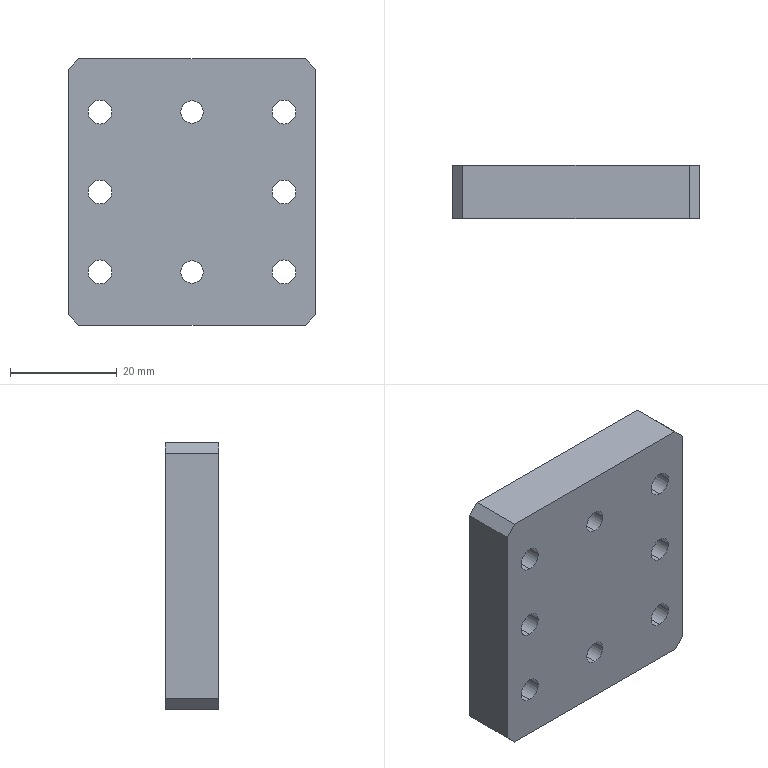Part | SolidWorks | features HoleWzd 2, Chamfer 1, Extrusion 1 | 1 solid | 44 faces | box 46.5 x 10 x 50 mm | volume 20990 mm3 | cylinder 28 | plane 16 | commonest cylinder face diameters 4.5 x12 8 x12 4.2 x4
STEP:
#1=CARTESIAN_POINT('',(0.,0.,-17.1));
#2=VERTEX_POINT('',#1);
#3=CARTESIAN_POINT('',(0.,0.,-12.9));
#4=VERTEX_POINT('',#3);
#5=CARTESIAN_POINT('',(0.,0.,-15.));
#6=DIRECTION('',(0.,1.,0.));
#7=DIRECTION('',(0.,0.,1.));
#8=AXIS2_PLACEMENT_3D('',#5,#6,#7);
#9=CIRCLE('',#8,2.1);
#10=EDGE_CURVE('',#2,#4,#9,.T.);
#11=ORIENTED_EDGE('',*,*,#10,.F.);
#12=CARTESIAN_POINT('',(0.,10.,-17.1));
#13=VERTEX_POINT('',#12);
#14=CARTESIAN_POINT('',(0.,10.,-17.1));
#15=DIRECTION('',(0.,1.,0.));
#16=VECTOR('',#15,1000.);
#17=LINE('',#14,#16);
#18=EDGE_CURVE('',#2,#13,#17,.T.);
#19=ORIENTED_EDGE('',*,*,#18,.T.);
#20=CARTESIAN_POINT('',(0.,10.,-12.9));
#21=VERTEX_POINT('',#20);
#22=CARTESIAN_POINT('',(0.,10.,-15.));
#23=DIRECTION('',(0.,1.,0.));
#24=DIRECTION('',(0.,0.,1.));
#25=AXIS2_PLACEMENT_3D('',#22,#23,#24);
#26=CIRCLE('',#25,2.1);
#27=EDGE_CURVE('',#13,#21,#26,.T.);
#28=ORIENTED_EDGE('',*,*,#27,.T.);
#29=CARTESIAN_POINT('',(0.,10.,-12.9));
#30=DIRECTION('',(0.,1.,0.));
#31=VECTOR('',#30,1000.);
#32=LINE('',#29,#31);
#33=EDGE_CURVE('',#4,#21,#32,.T.);
#34=ORIENTED_EDGE('',*,*,#33,.F.);
#35=EDGE_LOOP('',(#11,#19,#28,#34));
#36=FACE_OUTER_BOUND('',#35,.T.);
#37=CARTESIAN_POINT('',(0.,10.,-15.));
#38=DIRECTION('',(0.,1.,0.));
#39=DIRECTION('',(0.,0.,1.));
#40=AXIS2_PLACEMENT_3D('',#37,#38,#39);
#41=CYLINDRICAL_SURFACE('',#40,2.1);
#42=ADVANCED_FACE('',(#36),#41,.F.);
#43=CARTESIAN_POINT('',(0.,0.,12.9));
#44=VERTEX_POINT('',#43);
#45=CARTESIAN_POINT('',(0.,0.,17.1));
#46=VERTEX_POINT('',#45);
#47=CARTESIAN_POINT('',(0.,0.,15.));
#48=DIRECTION('',(0.,1.,0.));
#49=DIRECTION('',(0.,0.,1.));
#50=AXIS2_PLACEMENT_3D('',#47,#48,#49);
#51=CIRCLE('',#50,2.1);
#52=EDGE_CURVE('',#44,#46,#51,.T.);
#53=ORIENTED_EDGE('',*,*,#52,.F.);
#54=CARTESIAN_POINT('',(0.,10.,12.9));
#55=VERTEX_POINT('',#54);
#56=CARTESIAN_POINT('',(0.,10.,12.9));
#57=DIRECTION('',(0.,1.,0.));
#58=VECTOR('',#57,1000.);
#59=LINE('',#56,#58);
#60=EDGE_CURVE('',#44,#55,#59,.T.);
#61=ORIENTED_EDGE('',*,*,#60,.T.);
#62=CARTESIAN_POINT('',(0.,10.,17.1));
#63=VERTEX_POINT('',#62);
#64=CARTESIAN_POINT('',(0.,10.,15.));
#65=DIRECTION('',(0.,1.,0.));
#66=DIRECTION('',(0.,0.,1.));
#67=AXIS2_PLACEMENT_3D('',#64,#65,#66);
#68=CIRCLE('',#67,2.1);
#69=EDGE_CURVE('',#55,#63,#68,.T.);
#70=ORIENTED_EDGE('',*,*,#69,.T.);
#71=CARTESIAN_POINT('',(0.,10.,17.1));
#72=DIRECTION('',(0.,1.,0.));
#73=VECTOR('',#72,1000.);
#74=LINE('',#71,#73);
#75=EDGE_CURVE('',#46,#63,#74,.T.);
#76=ORIENTED_EDGE('',*,*,#75,.F.);
#77=EDGE_LOOP('',(#53,#61,#70,#76));
#78=FACE_OUTER_BOUND('',#77,.T.);
#79=CARTESIAN_POINT('',(0.,10.,15.));
#80=DIRECTION('',(0.,1.,0.));
#81=DIRECTION('',(0.,0.,1.));
#82=AXIS2_PLACEMENT_3D('',#79,#80,#81);
#83=CYLINDRICAL_SURFACE('',#82,2.1);
#84=ADVANCED_FACE('',(#78),#83,.F.);
#85=CARTESIAN_POINT('',(17.25,5.4,11.));
#86=VERTEX_POINT('',#85);
#87=CARTESIAN_POINT('',(17.25,5.4,19.));
#88=VERTEX_POINT('',#87);
#89=CARTESIAN_POINT('',(17.25,5.4,15.));
#90=DIRECTION('',(0.,1.,0.));
#91=DIRECTION('',(0.,0.,1.));
#92=AXIS2_PLACEMENT_3D('',#89,#90,#91);
#93=CIRCLE('',#92,4.);
#94=EDGE_CURVE('',#86,#88,#93,.T.);
#95=ORIENTED_EDGE('',*,*,#94,.F.);
#96=CARTESIAN_POINT('',(17.25,10.,11.));
#97=VERTEX_POINT('',#96);
#98=CARTESIAN_POINT('',(17.25,10.,11.));
#99=DIRECTION('',(0.,1.,0.));
#100=VECTOR('',#99,1000.);
#101=LINE('',#98,#100);
#102=EDGE_CURVE('',#86,#97,#101,.T.);
#103=ORIENTED_EDGE('',*,*,#102,.T.);
#104=CARTESIAN_POINT('',(17.25,10.,19.));
#105=VERTEX_POINT('',#104);
#106=CARTESIAN_POINT('',(17.25,10.,15.));
#107=DIRECTION('',(0.,1.,0.));
#108=DIRECTION('',(0.,0.,1.));
#109=AXIS2_PLACEMENT_3D('',#106,#107,#108);
#110=CIRCLE('',#109,4.);
#111=EDGE_CURVE('',#97,#105,#110,.T.);
#112=ORIENTED_EDGE('',*,*,#111,.T.);
#113=CARTESIAN_POINT('',(17.25,10.,19.));
#114=DIRECTION('',(0.,1.,0.));
#115=VECTOR('',#114,1000.);
#116=LINE('',#113,#115);
#117=EDGE_CURVE('',#88,#105,#116,.T.);
#118=ORIENTED_EDGE('',*,*,#117,.F.);
#119=EDGE_LOOP('',(#95,#103,#112,#118));
#120=FACE_OUTER_BOUND('',#119,.T.);
#121=CARTESIAN_POINT('',(17.25,10.,15.));
#122=DIRECTION('',(0.,1.,0.));
#123=DIRECTION('',(0.,0.,1.));
#124=AXIS2_PLACEMENT_3D('',#121,#122,#123);
#125=CYLINDRICAL_SURFACE('',#124,4.);
#126=ADVANCED_FACE('',(#120),#125,.F.);
#127=CARTESIAN_POINT('',(17.25,0.,12.75));
#128=VERTEX_POINT('',#127);
#129=CARTESIAN_POINT('',(17.25,0.,17.25));
#130=VERTEX_POINT('',#129);
#131=CARTESIAN_POINT('',(17.25,0.,15.));
#132=DIRECTION('',(0.,1.,0.));
#133=DIRECTION('',(0.,0.,1.));
#134=AXIS2_PLACEMENT_3D('',#131,#132,#133);
#135=CIRCLE('',#134,2.25);
#136=EDGE_CURVE('',#128,#130,#135,.T.);
#137=ORIENTED_EDGE('',*,*,#136,.F.);
#138=CARTESIAN_POINT('',(17.25,5.4,12.75));
#139=VERTEX_POINT('',#138);
#140=CARTESIAN_POINT('',(17.25,10.,12.75));
#141=DIRECTION('',(0.,1.,0.));
#142=VECTOR('',#141,1000.);
#143=LINE('',#140,#142);
#144=EDGE_CURVE('',#128,#139,#143,.T.);
#145=ORIENTED_EDGE('',*,*,#144,.T.);
#146=CARTESIAN_POINT('',(17.25,5.4,17.25));
#147=VERTEX_POINT('',#146);
#148=CARTESIAN_POINT('',(17.25,5.4,15.));
#149=DIRECTION('',(0.,1.,0.));
#150=DIRECTION('',(0.,0.,1.));
#151=AXIS2_PLACEMENT_3D('',#148,#149,#150);
#152=CIRCLE('',#151,2.25);
#153=EDGE_CURVE('',#139,#147,#152,.T.);
#154=ORIENTED_EDGE('',*,*,#153,.T.);
#155=CARTESIAN_POINT('',(17.25,10.,17.25));
#156=DIRECTION('',(0.,1.,0.));
#157=VECTOR('',#156,1000.);
#158=LINE('',#155,#157);
#159=EDGE_CURVE('',#130,#147,#158,.T.);
#160=ORIENTED_EDGE('',*,*,#159,.F.);
#161=EDGE_LOOP('',(#137,#145,#154,#160));
#162=FACE_OUTER_BOUND('',#161,.T.);
#163=CARTESIAN_POINT('',(17.25,10.,15.));
#164=DIRECTION('',(0.,1.,0.));
#165=DIRECTION('',(0.,0.,1.));
#166=AXIS2_PLACEMENT_3D('',#163,#164,#165);
#167=CYLINDRICAL_SURFACE('',#166,2.25);
#168=ADVANCED_FACE('',(#162),#167,.F.);
#169=CARTESIAN_POINT('',(17.25,5.4,-4.));
#170=VERTEX_POINT('',#169);
#171=CARTESIAN_POINT('',(17.25,5.4,4.));
#172=VERTEX_POINT('',#171);
#173=CARTESIAN_POINT('',(17.25,5.4,0.));
#174=DIRECTION('',(0.,1.,0.));
#175=DIRECTION('',(0.,0.,1.));
#176=AXIS2_PLACEMENT_3D('',#173,#174,#175);
#177=CIRCLE('',#176,4.);
#178=EDGE_CURVE('',#170,#172,#177,.T.);
#179=ORIENTED_EDGE('',*,*,#178,.F.);
#180=CARTESIAN_POINT('',(17.25,10.,-4.));
#181=VERTEX_POINT('',#180);
#182=CARTESIAN_POINT('',(17.25,10.,-4.));
#183=DIRECTION('',(0.,1.,0.));
#184=VECTOR('',#183,1000.);
#185=LINE('',#182,#184);
#186=EDGE_CURVE('',#170,#181,#185,.T.);
#187=ORIENTED_EDGE('',*,*,#186,.T.);
#188=CARTESIAN_POINT('',(17.25,10.,4.));
#189=VERTEX_POINT('',#188);
#190=CARTESIAN_POINT('',(17.25,10.,0.));
#191=DIRECTION('',(0.,1.,0.));
#192=DIRECTION('',(0.,0.,1.));
#193=AXIS2_PLACEMENT_3D('',#190,#191,#192);
#194=CIRCLE('',#193,4.);
#195=EDGE_CURVE('',#181,#189,#194,.T.);
#196=ORIENTED_EDGE('',*,*,#195,.T.);
#197=CARTESIAN_POINT('',(17.25,10.,4.));
#198=DIRECTION('',(0.,1.,0.));
#199=VECTOR('',#198,1000.);
#200=LINE('',#197,#199);
#201=EDGE_CURVE('',#172,#189,#200,.T.);
#202=ORIENTED_EDGE('',*,*,#201,.F.);
#203=EDGE_LOOP('',(#179,#187,#196,#202));
#204=FACE_OUTER_BOUND('',#203,.T.);
#205=CARTESIAN_POINT('',(17.25,10.,0.));
#206=DIRECTION('',(0.,1.,0.));
#207=DIRECTION('',(0.,0.,1.));
#208=AXIS2_PLACEMENT_3D('',#205,#206,#207);
#209=CYLINDRICAL_SURFACE('',#208,4.);
#210=ADVANCED_FACE('',(#204),#209,.F.);
#211=CARTESIAN_POINT('',(17.25,0.,-2.25));
#212=VERTEX_POINT('',#211);
#213=CARTESIAN_POINT('',(17.25,0.,2.25));
#214=VERTEX_POINT('',#213);
#215=CARTESIAN_POINT('',(17.25,0.,0.));
#216=DIRECTION('',(0.,1.,0.));
#217=DIRECTION('',(0.,0.,1.));
#218=AXIS2_PLACEMENT_3D('',#215,#216,#217);
#219=CIRCLE('',#218,2.25);
#220=EDGE_CURVE('',#212,#214,#219,.T.);
#221=ORIENTED_EDGE('',*,*,#220,.F.);
#222=CARTESIAN_POINT('',(17.25,5.4,-2.25));
#223=VERTEX_POINT('',#222);
#224=CARTESIAN_POINT('',(17.25,10.,-2.25));
#225=DIRECTION('',(0.,1.,0.));
#226=VECTOR('',#225,1000.);
#227=LINE('',#224,#226);
#228=EDGE_CURVE('',#212,#223,#227,.T.);
#229=ORIENTED_EDGE('',*,*,#228,.T.);
#230=CARTESIAN_POINT('',(17.25,5.4,2.25));
#231=VERTEX_POINT('',#230);
#232=CARTESIAN_POINT('',(17.25,5.4,0.));
#233=DIRECTION('',(0.,1.,0.));
#234=DIRECTION('',(0.,0.,1.));
#235=AXIS2_PLACEMENT_3D('',#232,#233,#234);
#236=CIRCLE('',#235,2.25);
#237=EDGE_CURVE('',#223,#231,#236,.T.);
#238=ORIENTED_EDGE('',*,*,#237,.T.);
#239=CARTESIAN_POINT('',(17.25,10.,2.25));
#240=DIRECTION('',(0.,1.,0.));
#241=VECTOR('',#240,1000.);
#242=LINE('',#239,#241);
#243=EDGE_CURVE('',#214,#231,#242,.T.);
#244=ORIENTED_EDGE('',*,*,#243,.F.);
#245=EDGE_LOOP('',(#221,#229,#238,#244));
#246=FACE_OUTER_BOUND('',#245,.T.);
#247=CARTESIAN_POINT('',(17.25,10.,0.));
#248=DIRECTION('',(0.,1.,0.));
#249=DIRECTION('',(0.,0.,1.));
#250=AXIS2_PLACEMENT_3D('',#247,#248,#249);
#251=CYLINDRICAL_SURFACE('',#250,2.25);
#252=ADVANCED_FACE('',(#246),#251,.F.);
#253=CARTESIAN_POINT('',(17.25,5.4,-19.));
#254=VERTEX_POINT('',#253);
#255=CARTESIAN_POINT('',(17.25,5.4,-11.));
#256=VERTEX_POINT('',#255);
#257=CARTESIAN_POINT('',(17.25,5.4,-15.));
#258=DIRECTION('',(0.,1.,0.));
#259=DIRECTION('',(0.,0.,1.));
#260=AXIS2_PLACEMENT_3D('',#257,#258,#259);
#261=CIRCLE('',#260,4.);
#262=EDGE_CURVE('',#254,#256,#261,.T.);
#263=ORIENTED_EDGE('',*,*,#262,.F.);
#264=CARTESIAN_POINT('',(17.25,10.,-19.));
#265=VERTEX_POINT('',#264);
#266=CARTESIAN_POINT('',(17.25,10.,-19.));
#267=DIRECTION('',(0.,1.,0.));
#268=VECTOR('',#267,1000.);
#269=LINE('',#266,#268);
#270=EDGE_CURVE('',#254,#265,#269,.T.);
#271=ORIENTED_EDGE('',*,*,#270,.T.);
#272=CARTESIAN_POINT('',(17.25,10.,-11.));
#273=VERTEX_POINT('',#272);
#274=CARTESIAN_POINT('',(17.25,10.,-15.));
#275=DIRECTION('',(0.,1.,0.));
#276=DIRECTION('',(0.,0.,1.));
#277=AXIS2_PLACEMENT_3D('',#274,#275,#276);
#278=CIRCLE('',#277,4.);
#279=EDGE_CURVE('',#265,#273,#278,.T.);
#280=ORIENTED_EDGE('',*,*,#279,.T.);
#281=CARTESIAN_POINT('',(17.25,10.,-11.));
#282=DIRECTION('',(0.,1.,0.));
#283=VECTOR('',#282,1000.);
#284=LINE('',#281,#283);
#285=EDGE_CURVE('',#256,#273,#284,.T.);
#286=ORIENTED_EDGE('',*,*,#285,.F.);
#287=EDGE_LOOP('',(#263,#271,#280,#286));
#288=FACE_OUTER_BOUND('',#287,.T.);
#289=CARTESIAN_POINT('',(17.25,10.,-15.));
#290=DIRECTION('',(0.,1.,0.));
#291=DIRECTION('',(0.,0.,1.));
#292=AXIS2_PLACEMENT_3D('',#289,#290,#291);
#293=CYLINDRICAL_SURFACE('',#292,4.);
#294=ADVANCED_FACE('',(#288),#293,.F.);
#295=CARTESIAN_POINT('',(17.25,0.,-17.25));
#296=VERTEX_POINT('',#295);
#297=CARTESIAN_POINT('',(17.25,0.,-12.75));
#298=VERTEX_POINT('',#297);
#299=CARTESIAN_POINT('',(17.25,0.,-15.));
#300=DIRECTION('',(0.,1.,0.));
#301=DIRECTION('',(0.,0.,1.));
#302=AXIS2_PLACEMENT_3D('',#299,#300,#301);
#303=CIRCLE('',#302,2.25);
#304=EDGE_CURVE('',#296,#298,#303,.T.);
#305=ORIENTED_EDGE('',*,*,#304,.F.);
#306=CARTESIAN_POINT('',(17.25,5.4,-17.25));
#307=VERTEX_POINT('',#306);
#308=CARTESIAN_POINT('',(17.25,10.,-17.25));
#309=DIRECTION('',(0.,1.,0.));
#310=VECTOR('',#309,1000.);
#311=LINE('',#308,#310);
#312=EDGE_CURVE('',#296,#307,#311,.T.);
#313=ORIENTED_EDGE('',*,*,#312,.T.);
#314=CARTESIAN_POINT('',(17.25,5.4,-12.75));
#315=VERTEX_POINT('',#314);
#316=CARTESIAN_POINT('',(17.25,5.4,-15.));
#317=DIRECTION('',(0.,1.,0.));
#318=DIRECTION('',(0.,0.,1.));
#319=AXIS2_PLACEMENT_3D('',#316,#317,#318);
#320=CIRCLE('',#319,2.25);
#321=EDGE_CURVE('',#307,#315,#320,.T.);
#322=ORIENTED_EDGE('',*,*,#321,.T.);
#323=CARTESIAN_POINT('',(17.25,10.,-12.75));
#324=DIRECTION('',(0.,1.,0.));
#325=VECTOR('',#324,1000.);
#326=LINE('',#323,#325);
#327=EDGE_CURVE('',#298,#315,#326,.T.);
#328=ORIENTED_EDGE('',*,*,#327,.F.);
#329=EDGE_LOOP('',(#305,#313,#322,#328));
#330=FACE_OUTER_BOUND('',#329,.T.);
#331=CARTESIAN_POINT('',(17.25,10.,-15.));
#332=DIRECTION('',(0.,1.,0.));
#333=DIRECTION('',(0.,0.,1.));
#334=AXIS2_PLACEMENT_3D('',#331,#332,#333);
#335=CYLINDRICAL_SURFACE('',#334,2.25);
#336=ADVANCED_FACE('',(#330),#335,.F.);
#337=CARTESIAN_POINT('',(-17.25,5.4,-19.));
#338=VERTEX_POINT('',#337);
#339=CARTESIAN_POINT('',(-17.25,5.4,-11.));
#340=VERTEX_POINT('',#339);
#341=CARTESIAN_POINT('',(-17.25,5.4,-15.));
#342=DIRECTION('',(0.,1.,0.));
#343=DIRECTION('',(0.,0.,1.));
#344=AXIS2_PLACEMENT_3D('',#341,#342,#343);
#345=CIRCLE('',#344,4.);
#346=EDGE_CURVE('',#338,#340,#345,.T.);
#347=ORIENTED_EDGE('',*,*,#346,.F.);
#348=CARTESIAN_POINT('',(-17.25,10.,-19.));
#349=VERTEX_POINT('',#348);
#350=CARTESIAN_POINT('',(-17.25,10.,-19.));
#351=DIRECTION('',(0.,1.,0.));
#352=VECTOR('',#351,1000.);
#353=LINE('',#350,#352);
#354=EDGE_CURVE('',#338,#349,#353,.T.);
#355=ORIENTED_EDGE('',*,*,#354,.T.);
#356=CARTESIAN_POINT('',(-17.25,10.,-11.));
#357=VERTEX_POINT('',#356);
#358=CARTESIAN_POINT('',(-17.25,10.,-15.));
#359=DIRECTION('',(0.,1.,0.));
#360=DIRECTION('',(0.,0.,1.));
#361=AXIS2_PLACEMENT_3D('',#358,#359,#360);
#362=CIRCLE('',#361,4.);
#363=EDGE_CURVE('',#349,#357,#362,.T.);
#364=ORIENTED_EDGE('',*,*,#363,.T.);
#365=CARTESIAN_POINT('',(-17.25,10.,-11.));
#366=DIRECTION('',(0.,1.,0.));
#367=VECTOR('',#366,1000.);
#368=LINE('',#365,#367);
#369=EDGE_CURVE('',#340,#357,#368,.T.);
#370=ORIENTED_EDGE('',*,*,#369,.F.);
#371=EDGE_LOOP('',(#347,#355,#364,#370));
#372=FACE_OUTER_BOUND('',#371,.T.);
#373=CARTESIAN_POINT('',(-17.25,10.,-15.));
#374=DIRECTION('',(0.,1.,0.));
#375=DIRECTION('',(0.,0.,1.));
#376=AXIS2_PLACEMENT_3D('',#373,#374,#375);
#377=CYLINDRICAL_SURFACE('',#376,4.);
#378=ADVANCED_FACE('',(#372),#377,.F.);
#379=CARTESIAN_POINT('',(-17.25,0.,-17.25));
#380=VERTEX_POINT('',#379);
#381=CARTESIAN_POINT('',(-17.25,0.,-12.75));
#382=VERTEX_POINT('',#381);
#383=CARTESIAN_POINT('',(-17.25,0.,-15.));
#384=DIRECTION('',(0.,1.,0.));
#385=DIRECTION('',(0.,0.,1.));
#386=AXIS2_PLACEMENT_3D('',#383,#384,#385);
#387=CIRCLE('',#386,2.25);
#388=EDGE_CURVE('',#380,#382,#387,.T.);
#389=ORIENTED_EDGE('',*,*,#388,.F.);
#390=CARTESIAN_POINT('',(-17.25,5.4,-17.25));
#391=VERTEX_POINT('',#390);
#392=CARTESIAN_POINT('',(-17.25,10.,-17.25));
#393=DIRECTION('',(0.,1.,0.));
#394=VECTOR('',#393,1000.);
#395=LINE('',#392,#394);
#396=EDGE_CURVE('',#380,#391,#395,.T.);
#397=ORIENTED_EDGE('',*,*,#396,.T.);
#398=CARTESIAN_POINT('',(-17.25,5.4,-12.75));
#399=VERTEX_POINT('',#398);
#400=CARTESIAN_POINT('',(-17.25,5.4,-15.));
#401=DIRECTION('',(0.,1.,0.));
#402=DIRECTION('',(0.,0.,1.));
#403=AXIS2_PLACEMENT_3D('',#400,#401,#402);
#404=CIRCLE('',#403,2.25);
#405=EDGE_CURVE('',#391,#399,#404,.T.);
#406=ORIENTED_EDGE('',*,*,#405,.T.);
#407=CARTESIAN_POINT('',(-17.25,10.,-12.75));
#408=DIRECTION('',(0.,1.,0.));
#409=VECTOR('',#408,1000.);
#410=LINE('',#407,#409);
#411=EDGE_CURVE('',#382,#399,#410,.T.);
#412=ORIENTED_EDGE('',*,*,#411,.F.);
#413=EDGE_LOOP('',(#389,#397,#406,#412));
#414=FACE_OUTER_BOUND('',#413,.T.);
#415=CARTESIAN_POINT('',(-17.25,10.,-15.));
#416=DIRECTION('',(0.,1.,0.));
#417=DIRECTION('',(0.,0.,1.));
#418=AXIS2_PLACEMENT_3D('',#415,#416,#417);
#419=CYLINDRICAL_SURFACE('',#418,2.25);
#420=ADVANCED_FACE('',(#414),#419,.F.);
#421=CARTESIAN_POINT('',(-17.25,5.4,-4.));
#422=VERTEX_POINT('',#421);
#423=CARTESIAN_POINT('',(-17.25,5.4,4.));
#424=VERTEX_POINT('',#423);
#425=CARTESIAN_POINT('',(-17.25,5.4,0.));
#426=DIRECTION('',(0.,1.,0.));
#427=DIRECTION('',(0.,0.,1.));
#428=AXIS2_PLACEMENT_3D('',#425,#426,#427);
#429=CIRCLE('',#428,4.);
#430=EDGE_CURVE('',#422,#424,#429,.T.);
#431=ORIENTED_EDGE('',*,*,#430,.F.);
#432=CARTESIAN_POINT('',(-17.25,10.,-4.));
#433=VERTEX_POINT('',#432);
#434=CARTESIAN_POINT('',(-17.25,10.,-4.));
#435=DIRECTION('',(0.,1.,0.));
#436=VECTOR('',#435,1000.);
#437=LINE('',#434,#436);
#438=EDGE_CURVE('',#422,#433,#437,.T.);
#439=ORIENTED_EDGE('',*,*,#438,.T.);
#440=CARTESIAN_POINT('',(-17.25,10.,4.));
#441=VERTEX_POINT('',#440);
#442=CARTESIAN_POINT('',(-17.25,10.,0.));
#443=DIRECTION('',(0.,1.,0.));
#444=DIRECTION('',(0.,0.,1.));
#445=AXIS2_PLACEMENT_3D('',#442,#443,#444);
#446=CIRCLE('',#445,4.);
#447=EDGE_CURVE('',#433,#441,#446,.T.);
#448=ORIENTED_EDGE('',*,*,#447,.T.);
#449=CARTESIAN_POINT('',(-17.25,10.,4.));
#450=DIRECTION('',(0.,1.,0.));
#451=VECTOR('',#450,1000.);
#452=LINE('',#449,#451);
#453=EDGE_CURVE('',#424,#441,#452,.T.);
#454=ORIENTED_EDGE('',*,*,#453,.F.);
#455=EDGE_LOOP('',(#431,#439,#448,#454));
#456=FACE_OUTER_BOUND('',#455,.T.);
#457=CARTESIAN_POINT('',(-17.25,10.,0.));
#458=DIRECTION('',(0.,1.,0.));
#459=DIRECTION('',(0.,0.,1.));
#460=AXIS2_PLACEMENT_3D('',#457,#458,#459);
#461=CYLINDRICAL_SURFACE('',#460,4.);
#462=ADVANCED_FACE('',(#456),#461,.F.);
#463=CARTESIAN_POINT('',(-17.25,0.,-2.25));
#464=VERTEX_POINT('',#463);
#465=CARTESIAN_POINT('',(-17.25,0.,2.25));
#466=VERTEX_POINT('',#465);
#467=CARTESIAN_POINT('',(-17.25,0.,0.));
#468=DIRECTION('',(0.,1.,0.));
#469=DIRECTION('',(0.,0.,1.));
#470=AXIS2_PLACEMENT_3D('',#467,#468,#469);
#471=CIRCLE('',#470,2.25);
#472=EDGE_CURVE('',#464,#466,#471,.T.);
#473=ORIENTED_EDGE('',*,*,#472,.F.);
#474=CARTESIAN_POINT('',(-17.25,5.4,-2.25));
#475=VERTEX_POINT('',#474);
#476=CARTESIAN_POINT('',(-17.25,10.,-2.25));
#477=DIRECTION('',(0.,1.,0.));
#478=VECTOR('',#477,1000.);
#479=LINE('',#476,#478);
#480=EDGE_CURVE('',#464,#475,#479,.T.);
#481=ORIENTED_EDGE('',*,*,#480,.T.);
#482=CARTESIAN_POINT('',(-17.25,5.4,2.25));
#483=VERTEX_POINT('',#482);
#484=CARTESIAN_POINT('',(-17.25,5.4,0.));
#485=DIRECTION('',(0.,1.,0.));
#486=DIRECTION('',(0.,0.,1.));
#487=AXIS2_PLACEMENT_3D('',#484,#485,#486);
#488=CIRCLE('',#487,2.25);
#489=EDGE_CURVE('',#475,#483,#488,.T.);
#490=ORIENTED_EDGE('',*,*,#489,.T.);
#491=CARTESIAN_POINT('',(-17.25,10.,2.25));
#492=DIRECTION('',(0.,1.,0.));
#493=VECTOR('',#492,1000.);
#494=LINE('',#491,#493);
#495=EDGE_CURVE('',#466,#483,#494,.T.);
#496=ORIENTED_EDGE('',*,*,#495,.F.);
#497=EDGE_LOOP('',(#473,#481,#490,#496));
#498=FACE_OUTER_BOUND('',#497,.T.);
#499=CARTESIAN_POINT('',(-17.25,10.,0.));
#500=DIRECTION('',(0.,1.,0.));
#501=DIRECTION('',(0.,0.,1.));
#502=AXIS2_PLACEMENT_3D('',#499,#500,#501);
#503=CYLINDRICAL_SURFACE('',#502,2.25);
#504=ADVANCED_FACE('',(#498),#503,.F.);
#505=CARTESIAN_POINT('',(-17.25,5.4,11.));
#506=VERTEX_POINT('',#505);
#507=CARTESIAN_POINT('',(-17.25,5.4,19.));
#508=VERTEX_POINT('',#507);
#509=CARTESIAN_POINT('',(-17.25,5.4,15.));
#510=DIRECTION('',(0.,1.,0.));
#511=DIRECTION('',(0.,0.,1.));
#512=AXIS2_PLACEMENT_3D('',#509,#510,#511);
#513=CIRCLE('',#512,4.);
#514=EDGE_CURVE('',#506,#508,#513,.T.);
#515=ORIENTED_EDGE('',*,*,#514,.F.);
#516=CARTESIAN_POINT('',(-17.25,10.,11.));
#517=VERTEX_POINT('',#516);
#518=CARTESIAN_POINT('',(-17.25,10.,11.));
#519=DIRECTION('',(0.,1.,0.));
#520=VECTOR('',#519,1000.);
#521=LINE('',#518,#520);
#522=EDGE_CURVE('',#506,#517,#521,.T.);
#523=ORIENTED_EDGE('',*,*,#522,.T.);
#524=CARTESIAN_POINT('',(-17.25,10.,19.));
#525=VERTEX_POINT('',#524);
#526=CARTESIAN_POINT('',(-17.25,10.,15.));
#527=DIRECTION('',(0.,1.,0.));
#528=DIRECTION('',(0.,0.,1.));
#529=AXIS2_PLACEMENT_3D('',#526,#527,#528);
#530=CIRCLE('',#529,4.);
#531=EDGE_CURVE('',#517,#525,#530,.T.);
#532=ORIENTED_EDGE('',*,*,#531,.T.);
#533=CARTESIAN_POINT('',(-17.25,10.,19.));
#534=DIRECTION('',(0.,1.,0.));
#535=VECTOR('',#534,1000.);
#536=LINE('',#533,#535);
#537=EDGE_CURVE('',#508,#525,#536,.T.);
#538=ORIENTED_EDGE('',*,*,#537,.F.);
#539=EDGE_LOOP('',(#515,#523,#532,#538));
#540=FACE_OUTER_BOUND('',#539,.T.);
#541=CARTESIAN_POINT('',(-17.25,10.,15.));
#542=DIRECTION('',(0.,1.,0.));
#543=DIRECTION('',(0.,0.,1.));
#544=AXIS2_PLACEMENT_3D('',#541,#542,#543);
#545=CYLINDRICAL_SURFACE('',#544,4.);
#546=ADVANCED_FACE('',(#540),#545,.F.);
#547=CARTESIAN_POINT('',(-17.25,0.,12.75));
#548=VERTEX_POINT('',#547);
#549=CARTESIAN_POINT('',(-17.25,0.,17.25));
#550=VERTEX_POINT('',#549);
#551=CARTESIAN_POINT('',(-17.25,0.,15.));
#552=DIRECTION('',(0.,1.,0.));
#553=DIRECTION('',(0.,0.,1.));
#554=AXIS2_PLACEMENT_3D('',#551,#552,#553);
#555=CIRCLE('',#554,2.25);
#556=EDGE_CURVE('',#548,#550,#555,.T.);
#557=ORIENTED_EDGE('',*,*,#556,.F.);
#558=CARTESIAN_POINT('',(-17.25,5.4,12.75));
#559=VERTEX_POINT('',#558);
#560=CARTESIAN_POINT('',(-17.25,10.,12.75));
#561=DIRECTION('',(0.,1.,0.));
#562=VECTOR('',#561,1000.);
#563=LINE('',#560,#562);
#564=EDGE_CURVE('',#548,#559,#563,.T.);
#565=ORIENTED_EDGE('',*,*,#564,.T.);
#566=CARTESIAN_POINT('',(-17.25,5.4,17.25));
#567=VERTEX_POINT('',#566);
#568=CARTESIAN_POINT('',(-17.25,5.4,15.));
#569=DIRECTION('',(0.,1.,0.));
#570=DIRECTION('',(0.,0.,1.));
#571=AXIS2_PLACEMENT_3D('',#568,#569,#570);
#572=CIRCLE('',#571,2.25);
#573=EDGE_CURVE('',#559,#567,#572,.T.);
#574=ORIENTED_EDGE('',*,*,#573,.T.);
#575=CARTESIAN_POINT('',(-17.25,10.,17.25));
#576=DIRECTION('',(0.,1.,0.));
#577=VECTOR('',#576,1000.);
#578=LINE('',#575,#577);
#579=EDGE_CURVE('',#550,#567,#578,.T.);
#580=ORIENTED_EDGE('',*,*,#579,.F.);
#581=EDGE_LOOP('',(#557,#565,#574,#580));
#582=FACE_OUTER_BOUND('',#581,.T.);
#583=CARTESIAN_POINT('',(-17.25,10.,15.));
#584=DIRECTION('',(0.,1.,0.));
#585=DIRECTION('',(0.,0.,1.));
#586=AXIS2_PLACEMENT_3D('',#583,#584,#585);
#587=CYLINDRICAL_SURFACE('',#586,2.25);
#588=ADVANCED_FACE('',(#582),#587,.F.);
#589=CARTESIAN_POINT('',(23.25,10.,23.));
#590=VERTEX_POINT('',#589);
#591=CARTESIAN_POINT('',(23.25,10.,-23.));
#592=VERTEX_POINT('',#591);
#593=CARTESIAN_POINT('',(23.25,10.,-25.));
#594=DIRECTION('',(0.,0.,-1.));
#595=VECTOR('',#594,1000.);
#596=LINE('',#593,#595);
#597=EDGE_CURVE('',#590,#592,#596,.T.);
#598=ORIENTED_EDGE('',*,*,#597,.F.);
#599=CARTESIAN_POINT('',(23.25,0.,23.));
#600=VERTEX_POINT('',#599);
#601=CARTESIAN_POINT('',(23.25,10.,23.));
#602=DIRECTION('',(0.,-1.,0.));
#603=VECTOR('',#602,1000.);
#604=LINE('',#601,#603);
#605=EDGE_CURVE('',#590,#600,#604,.T.);
#606=ORIENTED_EDGE('',*,*,#605,.T.);
#607=CARTESIAN_POINT('',(23.25,0.,-23.));
#608=VERTEX_POINT('',#607);
#609=CARTESIAN_POINT('',(23.25,0.,-25.));
#610=DIRECTION('',(0.,0.,-1.));
#611=VECTOR('',#610,1000.);
#612=LINE('',#609,#611);
#613=EDGE_CURVE('',#600,#608,#612,.T.);
#614=ORIENTED_EDGE('',*,*,#613,.T.);
#615=CARTESIAN_POINT('',(23.25,10.,-23.));
#616=DIRECTION('',(0.,1.,0.));
#617=VECTOR('',#616,1000.);
#618=LINE('',#615,#617);
#619=EDGE_CURVE('',#608,#592,#618,.T.);
#620=ORIENTED_EDGE('',*,*,#619,.T.);
#621=EDGE_LOOP('',(#598,#606,#614,#620));
#622=FACE_OUTER_BOUND('',#621,.T.);
#623=CARTESIAN_POINT('',(23.25,10.,-25.));
#624=DIRECTION('',(-1.,0.,0.));
#625=DIRECTION('',(0.,0.,1.));
#626=AXIS2_PLACEMENT_3D('',#623,#624,#625);
#627=PLANE('',#626);
#628=ADVANCED_FACE('',(#622),#627,.F.);
#629=CARTESIAN_POINT('',(21.25,0.,-25.));
#630=VERTEX_POINT('',#629);
#631=CARTESIAN_POINT('',(-21.25,0.,-25.));
#632=VERTEX_POINT('',#631);
#633=CARTESIAN_POINT('',(-23.25,0.,-25.));
#634=DIRECTION('',(-1.,0.,0.));
#635=VECTOR('',#634,1000.);
#636=LINE('',#633,#635);
#637=EDGE_CURVE('',#630,#632,#636,.T.);
#638=ORIENTED_EDGE('',*,*,#637,.T.);
#639=CARTESIAN_POINT('',(-21.25,10.,-25.));
#640=VERTEX_POINT('',#639);
#641=CARTESIAN_POINT('',(-21.25,10.,-25.));
#642=DIRECTION('',(0.,1.,0.));
#643=VECTOR('',#642,1000.);
#644=LINE('',#641,#643);
#645=EDGE_CURVE('',#632,#640,#644,.T.);
#646=ORIENTED_EDGE('',*,*,#645,.T.);
#647=CARTESIAN_POINT('',(21.25,10.,-25.));
#648=VERTEX_POINT('',#647);
#649=CARTESIAN_POINT('',(-23.25,10.,-25.));
#650=DIRECTION('',(-1.,0.,0.));
#651=VECTOR('',#650,1000.);
#652=LINE('',#649,#651);
#653=EDGE_CURVE('',#648,#640,#652,.T.);
#654=ORIENTED_EDGE('',*,*,#653,.F.);
#655=CARTESIAN_POINT('',(21.25,10.,-25.));
#656=DIRECTION('',(0.,-1.,0.));
#657=VECTOR('',#656,1000.);
#658=LINE('',#655,#657);
#659=EDGE_CURVE('',#648,#630,#658,.T.);
#660=ORIENTED_EDGE('',*,*,#659,.T.);
#661=EDGE_LOOP('',(#638,#646,#654,#660));
#662=FACE_OUTER_BOUND('',#661,.T.);
#663=CARTESIAN_POINT('',(-23.25,10.,-25.));
#664=DIRECTION('',(0.,0.,1.));
#665=DIRECTION('',(1.,0.,0.));
#666=AXIS2_PLACEMENT_3D('',#663,#664,#665);
#667=PLANE('',#666);
#668=ADVANCED_FACE('',(#662),#667,.F.);
#669=CARTESIAN_POINT('',(-23.25,0.,-23.));
#670=VERTEX_POINT('',#669);
#671=CARTESIAN_POINT('',(-23.25,0.,23.));
#672=VERTEX_POINT('',#671);
#673=CARTESIAN_POINT('',(-23.25,0.,-25.));
#674=DIRECTION('',(0.,0.,1.));
#675=VECTOR('',#674,1000.);
#676=LINE('',#673,#675);
#677=EDGE_CURVE('',#670,#672,#676,.T.);
#678=ORIENTED_EDGE('',*,*,#677,.T.);
#679=CARTESIAN_POINT('',(-23.25,10.,23.));
#680=VERTEX_POINT('',#679);
#681=CARTESIAN_POINT('',(-23.25,10.,23.));
#682=DIRECTION('',(0.,1.,0.));
#683=VECTOR('',#682,1000.);
#684=LINE('',#681,#683);
#685=EDGE_CURVE('',#672,#680,#684,.T.);
#686=ORIENTED_EDGE('',*,*,#685,.T.);
#687=CARTESIAN_POINT('',(-23.25,10.,-23.));
#688=VERTEX_POINT('',#687);
#689=CARTESIAN_POINT('',(-23.25,10.,-25.));
#690=DIRECTION('',(0.,0.,1.));
#691=VECTOR('',#690,1000.);
#692=LINE('',#689,#691);
#693=EDGE_CURVE('',#688,#680,#692,.T.);
#694=ORIENTED_EDGE('',*,*,#693,.F.);
#695=CARTESIAN_POINT('',(-23.25,10.,-23.));
#696=DIRECTION('',(0.,-1.,0.));
#697=VECTOR('',#696,1000.);
#698=LINE('',#695,#697);
#699=EDGE_CURVE('',#688,#670,#698,.T.);
#700=ORIENTED_EDGE('',*,*,#699,.T.);
#701=EDGE_LOOP('',(#678,#686,#694,#700));
#702=FACE_OUTER_BOUND('',#701,.T.);
#703=CARTESIAN_POINT('',(-23.25,10.,-25.));
#704=DIRECTION('',(1.,0.,0.));
#705=DIRECTION('',(0.,0.,-1.));
#706=AXIS2_PLACEMENT_3D('',#703,#704,#705);
#707=PLANE('',#706);
#708=ADVANCED_FACE('',(#702),#707,.F.);
#709=CARTESIAN_POINT('',(-21.25,0.,25.));
#710=VERTEX_POINT('',#709);
#711=CARTESIAN_POINT('',(21.25,0.,25.));
#712=VERTEX_POINT('',#711);
#713=CARTESIAN_POINT('',(-23.25,0.,25.));
#714=DIRECTION('',(1.,0.,0.));
#715=VECTOR('',#714,1000.);
#716=LINE('',#713,#715);
#717=EDGE_CURVE('',#710,#712,#716,.T.);
#718=ORIENTED_EDGE('',*,*,#717,.T.);
#719=CARTESIAN_POINT('',(21.25,10.,25.));
#720=VERTEX_POINT('',#719);
#721=CARTESIAN_POINT('',(21.25,10.,25.));
#722=DIRECTION('',(0.,1.,0.));
#723=VECTOR('',#722,1000.);
#724=LINE('',#721,#723);
#725=EDGE_CURVE('',#712,#720,#724,.T.);
#726=ORIENTED_EDGE('',*,*,#725,.T.);
#727=CARTESIAN_POINT('',(-21.25,10.,25.));
#728=VERTEX_POINT('',#727);
#729=CARTESIAN_POINT('',(-23.25,10.,25.));
#730=DIRECTION('',(1.,0.,0.));
#731=VECTOR('',#730,1000.);
#732=LINE('',#729,#731);
#733=EDGE_CURVE('',#728,#720,#732,.T.);
#734=ORIENTED_EDGE('',*,*,#733,.F.);
#735=CARTESIAN_POINT('',(-21.25,10.,25.));
#736=DIRECTION('',(0.,-1.,0.));
#737=VECTOR('',#736,1000.);
#738=LINE('',#735,#737);
#739=EDGE_CURVE('',#728,#710,#738,.T.);
#740=ORIENTED_EDGE('',*,*,#739,.T.);
#741=EDGE_LOOP('',(#718,#726,#734,#740));
#742=FACE_OUTER_BOUND('',#741,.T.);
#743=CARTESIAN_POINT('',(-23.25,10.,25.));
#744=DIRECTION('',(0.,0.,-1.));
#745=DIRECTION('',(-1.,0.,0.));
#746=AXIS2_PLACEMENT_3D('',#743,#744,#745);
#747=PLANE('',#746);
#748=ADVANCED_FACE('',(#742),#747,.F.);
#749=CARTESIAN_POINT('',(0.,10.,-15.));
#750=DIRECTION('',(0.,1.,0.));
#751=DIRECTION('',(0.,0.,1.));
#752=AXIS2_PLACEMENT_3D('',#749,#750,#751);
#753=CIRCLE('',#752,2.1);
#754=EDGE_CURVE('',#21,#13,#753,.T.);
#755=ORIENTED_EDGE('',*,*,#754,.F.);
#756=ORIENTED_EDGE('',*,*,#27,.F.);
#757=EDGE_LOOP('',(#755,#756));
#758=FACE_BOUND('',#757,.T.);
#759=CARTESIAN_POINT('',(0.,10.,15.));
#760=DIRECTION('',(0.,1.,0.));
#761=DIRECTION('',(0.,0.,1.));
#762=AXIS2_PLACEMENT_3D('',#759,#760,#761);
#763=CIRCLE('',#762,2.1);
#764=EDGE_CURVE('',#63,#55,#763,.T.);
#765=ORIENTED_EDGE('',*,*,#764,.F.);
#766=ORIENTED_EDGE('',*,*,#69,.F.);
#767=EDGE_LOOP('',(#765,#766));
#768=FACE_BOUND('',#767,.T.);
#769=CARTESIAN_POINT('',(17.25,10.,15.));
#770=DIRECTION('',(0.,1.,0.));
#771=DIRECTION('',(0.,0.,1.));
#772=AXIS2_PLACEMENT_3D('',#769,#770,#771);
#773=CIRCLE('',#772,4.);
#774=EDGE_CURVE('',#105,#97,#773,.T.);
#775=ORIENTED_EDGE('',*,*,#774,.F.);
#776=ORIENTED_EDGE('',*,*,#111,.F.);
#777=EDGE_LOOP('',(#775,#776));
#778=FACE_BOUND('',#777,.T.);
#779=CARTESIAN_POINT('',(17.25,10.,0.));
#780=DIRECTION('',(0.,1.,0.));
#781=DIRECTION('',(0.,0.,1.));
#782=AXIS2_PLACEMENT_3D('',#779,#780,#781);
#783=CIRCLE('',#782,4.);
#784=EDGE_CURVE('',#189,#181,#783,.T.);
#785=ORIENTED_EDGE('',*,*,#784,.F.);
#786=ORIENTED_EDGE('',*,*,#195,.F.);
#787=EDGE_LOOP('',(#785,#786));
#788=FACE_BOUND('',#787,.T.);
#789=CARTESIAN_POINT('',(17.25,10.,-15.));
#790=DIRECTION('',(0.,1.,0.));
#791=DIRECTION('',(0.,0.,1.));
#792=AXIS2_PLACEMENT_3D('',#789,#790,#791);
#793=CIRCLE('',#792,4.);
#794=EDGE_CURVE('',#273,#265,#793,.T.);
#795=ORIENTED_EDGE('',*,*,#794,.F.);
#796=ORIENTED_EDGE('',*,*,#279,.F.);
#797=EDGE_LOOP('',(#795,#796));
#798=FACE_BOUND('',#797,.T.);
#799=CARTESIAN_POINT('',(-17.25,10.,-15.));
#800=DIRECTION('',(0.,1.,0.));
#801=DIRECTION('',(0.,0.,1.));
#802=AXIS2_PLACEMENT_3D('',#799,#800,#801);
#803=CIRCLE('',#802,4.);
#804=EDGE_CURVE('',#357,#349,#803,.T.);
#805=ORIENTED_EDGE('',*,*,#804,.F.);
#806=ORIENTED_EDGE('',*,*,#363,.F.);
#807=EDGE_LOOP('',(#805,#806));
#808=FACE_BOUND('',#807,.T.);
#809=CARTESIAN_POINT('',(-17.25,10.,0.));
#810=DIRECTION('',(0.,1.,0.));
#811=DIRECTION('',(0.,0.,1.));
#812=AXIS2_PLACEMENT_3D('',#809,#810,#811);
#813=CIRCLE('',#812,4.);
#814=EDGE_CURVE('',#441,#433,#813,.T.);
#815=ORIENTED_EDGE('',*,*,#814,.F.);
#816=ORIENTED_EDGE('',*,*,#447,.F.);
#817=EDGE_LOOP('',(#815,#816));
#818=FACE_BOUND('',#817,.T.);
#819=CARTESIAN_POINT('',(-17.25,10.,15.));
#820=DIRECTION('',(0.,1.,0.));
#821=DIRECTION('',(0.,0.,1.));
#822=AXIS2_PLACEMENT_3D('',#819,#820,#821);
#823=CIRCLE('',#822,4.);
#824=EDGE_CURVE('',#525,#517,#823,.T.);
#825=ORIENTED_EDGE('',*,*,#824,.F.);
#826=ORIENTED_EDGE('',*,*,#531,.F.);
#827=EDGE_LOOP('',(#825,#826));
#828=FACE_BOUND('',#827,.T.);
#829=ORIENTED_EDGE('',*,*,#733,.T.);
#830=CARTESIAN_POINT('',(23.125,10.,23.125));
#831=DIRECTION('',(0.7071,0.,-0.7071));
#832=VECTOR('',#831,1000.);
#833=LINE('',#830,#832);
#834=EDGE_CURVE('',#720,#590,#833,.T.);
#835=ORIENTED_EDGE('',*,*,#834,.T.);
#836=ORIENTED_EDGE('',*,*,#597,.T.);
#837=CARTESIAN_POINT('',(23.125,10.,-23.125));
#838=DIRECTION('',(-0.7071,0.,-0.7071));
#839=VECTOR('',#838,1000.);
#840=LINE('',#837,#839);
#841=EDGE_CURVE('',#592,#648,#840,.T.);
#842=ORIENTED_EDGE('',*,*,#841,.T.);
#843=ORIENTED_EDGE('',*,*,#653,.T.);
#844=CARTESIAN_POINT('',(-23.125,10.,-23.125));
#845=DIRECTION('',(-0.7071,0.,0.7071));
#846=VECTOR('',#845,1000.);
#847=LINE('',#844,#846);
#848=EDGE_CURVE('',#640,#688,#847,.T.);
#849=ORIENTED_EDGE('',*,*,#848,.T.);
#850=ORIENTED_EDGE('',*,*,#693,.T.);
#851=CARTESIAN_POINT('',(-23.125,10.,23.125));
#852=DIRECTION('',(0.7071,0.,0.7071));
#853=VECTOR('',#852,1000.);
#854=LINE('',#851,#853);
#855=EDGE_CURVE('',#680,#728,#854,.T.);
#856=ORIENTED_EDGE('',*,*,#855,.T.);
#857=EDGE_LOOP('',(#829,#835,#836,#842,#843,#849,#850,#856));
#858=FACE_OUTER_BOUND('',#857,.T.);
#859=CARTESIAN_POINT('',(0.,10.,0.));
#860=DIRECTION('',(0.,1.,0.));
#861=DIRECTION('',(0.,0.,1.));
#862=AXIS2_PLACEMENT_3D('',#859,#860,#861);
#863=PLANE('',#862);
#864=ADVANCED_FACE('',(#758,#768,#778,#788,#798,#808,#818,#828,#858),#863,.T.);
#865=CARTESIAN_POINT('',(0.,0.,-15.));
#866=DIRECTION('',(0.,1.,0.));
#867=DIRECTION('',(0.,0.,1.));
#868=AXIS2_PLACEMENT_3D('',#865,#866,#867);
#869=CIRCLE('',#868,2.1);
#870=EDGE_CURVE('',#4,#2,#869,.T.);
#871=ORIENTED_EDGE('',*,*,#870,.T.);
#872=ORIENTED_EDGE('',*,*,#10,.T.);
#873=EDGE_LOOP('',(#871,#872));
#874=FACE_BOUND('',#873,.T.);
#875=CARTESIAN_POINT('',(0.,0.,15.));
#876=DIRECTION('',(0.,1.,0.));
#877=DIRECTION('',(0.,0.,1.));
#878=AXIS2_PLACEMENT_3D('',#875,#876,#877);
#879=CIRCLE('',#878,2.1);
#880=EDGE_CURVE('',#46,#44,#879,.T.);
#881=ORIENTED_EDGE('',*,*,#880,.T.);
#882=ORIENTED_EDGE('',*,*,#52,.T.);
#883=EDGE_LOOP('',(#881,#882));
#884=FACE_BOUND('',#883,.T.);
#885=CARTESIAN_POINT('',(17.25,0.,15.));
#886=DIRECTION('',(0.,1.,0.));
#887=DIRECTION('',(0.,0.,1.));
#888=AXIS2_PLACEMENT_3D('',#885,#886,#887);
#889=CIRCLE('',#888,2.25);
#890=EDGE_CURVE('',#130,#128,#889,.T.);
#891=ORIENTED_EDGE('',*,*,#890,.T.);
#892=ORIENTED_EDGE('',*,*,#136,.T.);
#893=EDGE_LOOP('',(#891,#892));
#894=FACE_BOUND('',#893,.T.);
#895=CARTESIAN_POINT('',(17.25,0.,0.));
#896=DIRECTION('',(0.,1.,0.));
#897=DIRECTION('',(0.,0.,1.));
#898=AXIS2_PLACEMENT_3D('',#895,#896,#897);
#899=CIRCLE('',#898,2.25);
#900=EDGE_CURVE('',#214,#212,#899,.T.);
#901=ORIENTED_EDGE('',*,*,#900,.T.);
#902=ORIENTED_EDGE('',*,*,#220,.T.);
#903=EDGE_LOOP('',(#901,#902));
#904=FACE_BOUND('',#903,.T.);
#905=CARTESIAN_POINT('',(17.25,0.,-15.));
#906=DIRECTION('',(0.,1.,0.));
#907=DIRECTION('',(0.,0.,1.));
#908=AXIS2_PLACEMENT_3D('',#905,#906,#907);
#909=CIRCLE('',#908,2.25);
#910=EDGE_CURVE('',#298,#296,#909,.T.);
#911=ORIENTED_EDGE('',*,*,#910,.T.);
#912=ORIENTED_EDGE('',*,*,#304,.T.);
#913=EDGE_LOOP('',(#911,#912));
#914=FACE_BOUND('',#913,.T.);
#915=CARTESIAN_POINT('',(-17.25,0.,-15.));
#916=DIRECTION('',(0.,1.,0.));
#917=DIRECTION('',(0.,0.,1.));
#918=AXIS2_PLACEMENT_3D('',#915,#916,#917);
#919=CIRCLE('',#918,2.25);
#920=EDGE_CURVE('',#382,#380,#919,.T.);
#921=ORIENTED_EDGE('',*,*,#920,.T.);
#922=ORIENTED_EDGE('',*,*,#388,.T.);
#923=EDGE_LOOP('',(#921,#922));
#924=FACE_BOUND('',#923,.T.);
#925=CARTESIAN_POINT('',(-17.25,0.,0.));
#926=DIRECTION('',(0.,1.,0.));
#927=DIRECTION('',(0.,0.,1.));
#928=AXIS2_PLACEMENT_3D('',#925,#926,#927);
#929=CIRCLE('',#928,2.25);
#930=EDGE_CURVE('',#466,#464,#929,.T.);
#931=ORIENTED_EDGE('',*,*,#930,.T.);
#932=ORIENTED_EDGE('',*,*,#472,.T.);
#933=EDGE_LOOP('',(#931,#932));
#934=FACE_BOUND('',#933,.T.);
#935=CARTESIAN_POINT('',(-17.25,0.,15.));
#936=DIRECTION('',(0.,1.,0.));
#937=DIRECTION('',(0.,0.,1.));
#938=AXIS2_PLACEMENT_3D('',#935,#936,#937);
#939=CIRCLE('',#938,2.25);
#940=EDGE_CURVE('',#550,#548,#939,.T.);
#941=ORIENTED_EDGE('',*,*,#940,.T.);
#942=ORIENTED_EDGE('',*,*,#556,.T.);
#943=EDGE_LOOP('',(#941,#942));
#944=FACE_BOUND('',#943,.T.);
#945=ORIENTED_EDGE('',*,*,#613,.F.);
#946=CARTESIAN_POINT('',(23.25,0.,23.));
#947=DIRECTION('',(-0.7071,0.,0.7071));
#948=VECTOR('',#947,1000.);
#949=LINE('',#946,#948);
#950=EDGE_CURVE('',#600,#712,#949,.T.);
#951=ORIENTED_EDGE('',*,*,#950,.T.);
#952=ORIENTED_EDGE('',*,*,#717,.F.);
#953=CARTESIAN_POINT('',(-21.25,0.,25.));
#954=DIRECTION('',(-0.7071,0.,-0.7071));
#955=VECTOR('',#954,1000.);
#956=LINE('',#953,#955);
#957=EDGE_CURVE('',#710,#672,#956,.T.);
#958=ORIENTED_EDGE('',*,*,#957,.T.);
#959=ORIENTED_EDGE('',*,*,#677,.F.);
#960=CARTESIAN_POINT('',(-23.25,0.,-23.));
#961=DIRECTION('',(0.7071,0.,-0.7071));
#962=VECTOR('',#961,1000.);
#963=LINE('',#960,#962);
#964=EDGE_CURVE('',#670,#632,#963,.T.);
#965=ORIENTED_EDGE('',*,*,#964,.T.);
#966=ORIENTED_EDGE('',*,*,#637,.F.);
#967=CARTESIAN_POINT('',(21.25,0.,-25.));
#968=DIRECTION('',(0.7071,0.,0.7071));
#969=VECTOR('',#968,1000.);
#970=LINE('',#967,#969);
#971=EDGE_CURVE('',#630,#608,#970,.T.);
#972=ORIENTED_EDGE('',*,*,#971,.T.);
#973=EDGE_LOOP('',(#945,#951,#952,#958,#959,#965,#966,#972));
#974=FACE_OUTER_BOUND('',#973,.T.);
#975=CARTESIAN_POINT('',(0.,0.,0.));
#976=DIRECTION('',(0.,1.,0.));
#977=DIRECTION('',(0.,0.,1.));
#978=AXIS2_PLACEMENT_3D('',#975,#976,#977);
#979=PLANE('',#978);
#980=ADVANCED_FACE('',(#874,#884,#894,#904,#914,#924,#934,#944,#974),#979,.F.);
#981=ORIENTED_EDGE('',*,*,#564,.F.);
#982=ORIENTED_EDGE('',*,*,#940,.F.);
#983=ORIENTED_EDGE('',*,*,#579,.T.);
#984=CARTESIAN_POINT('',(-17.25,5.4,15.));
#985=DIRECTION('',(0.,1.,0.));
#986=DIRECTION('',(0.,0.,1.));
#987=AXIS2_PLACEMENT_3D('',#984,#985,#986);
#988=CIRCLE('',#987,2.25);
#989=EDGE_CURVE('',#567,#559,#988,.T.);
#990=ORIENTED_EDGE('',*,*,#989,.T.);
#991=EDGE_LOOP('',(#981,#982,#983,#990));
#992=FACE_OUTER_BOUND('',#991,.T.);
#993=CARTESIAN_POINT('',(-17.25,10.,15.));
#994=DIRECTION('',(0.,1.,0.));
#995=DIRECTION('',(0.,0.,1.));
#996=AXIS2_PLACEMENT_3D('',#993,#994,#995);
#997=CYLINDRICAL_SURFACE('',#996,2.25);
#998=ADVANCED_FACE('',(#992),#997,.F.);
#999=ORIENTED_EDGE('',*,*,#989,.F.);
#1000=ORIENTED_EDGE('',*,*,#573,.F.);
#1001=EDGE_LOOP('',(#999,#1000));
#1002=FACE_BOUND('',#1001,.T.);
#1003=CARTESIAN_POINT('',(-17.25,5.4,15.));
#1004=DIRECTION('',(0.,1.,0.));
#1005=DIRECTION('',(0.,0.,1.));
#1006=AXIS2_PLACEMENT_3D('',#1003,#1004,#1005);
#1007=CIRCLE('',#1006,4.);
#1008=EDGE_CURVE('',#508,#506,#1007,.T.);
#1009=ORIENTED_EDGE('',*,*,#1008,.T.);
#1010=ORIENTED_EDGE('',*,*,#514,.T.);
#1011=EDGE_LOOP('',(#1009,#1010));
#1012=FACE_OUTER_BOUND('',#1011,.T.);
#1013=CARTESIAN_POINT('',(-15.,5.4,15.));
#1014=DIRECTION('',(0.,-1.,0.));
#1015=DIRECTION('',(0.,0.,-1.));
#1016=AXIS2_PLACEMENT_3D('',#1013,#1014,#1015);
#1017=PLANE('',#1016);
#1018=ADVANCED_FACE('',(#1002,#1012),#1017,.F.);
#1019=ORIENTED_EDGE('',*,*,#522,.F.);
#1020=ORIENTED_EDGE('',*,*,#1008,.F.);
#1021=ORIENTED_EDGE('',*,*,#537,.T.);
#1022=ORIENTED_EDGE('',*,*,#824,.T.);
#1023=EDGE_LOOP('',(#1019,#1020,#1021,#1022));
#1024=FACE_OUTER_BOUND('',#1023,.T.);
#1025=CARTESIAN_POINT('',(-17.25,10.,15.));
#1026=DIRECTION('',(0.,1.,0.));
#1027=DIRECTION('',(0.,0.,1.));
#1028=AXIS2_PLACEMENT_3D('',#1025,#1026,#1027);
#1029=CYLINDRICAL_SURFACE('',#1028,4.);
#1030=ADVANCED_FACE('',(#1024),#1029,.F.);
#1031=ORIENTED_EDGE('',*,*,#480,.F.);
#1032=ORIENTED_EDGE('',*,*,#930,.F.);
#1033=ORIENTED_EDGE('',*,*,#495,.T.);
#1034=CARTESIAN_POINT('',(-17.25,5.4,0.));
#1035=DIRECTION('',(0.,1.,0.));
#1036=DIRECTION('',(0.,0.,1.));
#1037=AXIS2_PLACEMENT_3D('',#1034,#1035,#1036);
#1038=CIRCLE('',#1037,2.25);
#1039=EDGE_CURVE('',#483,#475,#1038,.T.);
#1040=ORIENTED_EDGE('',*,*,#1039,.T.);
#1041=EDGE_LOOP('',(#1031,#1032,#1033,#1040));
#1042=FACE_OUTER_BOUND('',#1041,.T.);
#1043=CARTESIAN_POINT('',(-17.25,10.,0.));
#1044=DIRECTION('',(0.,1.,0.));
#1045=DIRECTION('',(0.,0.,1.));
#1046=AXIS2_PLACEMENT_3D('',#1043,#1044,#1045);
#1047=CYLINDRICAL_SURFACE('',#1046,2.25);
#1048=ADVANCED_FACE('',(#1042),#1047,.F.);
#1049=ORIENTED_EDGE('',*,*,#1039,.F.);
#1050=ORIENTED_EDGE('',*,*,#489,.F.);
#1051=EDGE_LOOP('',(#1049,#1050));
#1052=FACE_BOUND('',#1051,.T.);
#1053=CARTESIAN_POINT('',(-17.25,5.4,0.));
#1054=DIRECTION('',(0.,1.,0.));
#1055=DIRECTION('',(0.,0.,1.));
#1056=AXIS2_PLACEMENT_3D('',#1053,#1054,#1055);
#1057=CIRCLE('',#1056,4.);
#1058=EDGE_CURVE('',#424,#422,#1057,.T.);
#1059=ORIENTED_EDGE('',*,*,#1058,.T.);
#1060=ORIENTED_EDGE('',*,*,#430,.T.);
#1061=EDGE_LOOP('',(#1059,#1060));
#1062=FACE_OUTER_BOUND('',#1061,.T.);
#1063=CARTESIAN_POINT('',(-15.,5.4,0.));
#1064=DIRECTION('',(0.,-1.,0.));
#1065=DIRECTION('',(0.,0.,-1.));
#1066=AXIS2_PLACEMENT_3D('',#1063,#1064,#1065);
#1067=PLANE('',#1066);
#1068=ADVANCED_FACE('',(#1052,#1062),#1067,.F.);
#1069=ORIENTED_EDGE('',*,*,#438,.F.);
#1070=ORIENTED_EDGE('',*,*,#1058,.F.);
#1071=ORIENTED_EDGE('',*,*,#453,.T.);
#1072=ORIENTED_EDGE('',*,*,#814,.T.);
#1073=EDGE_LOOP('',(#1069,#1070,#1071,#1072));
#1074=FACE_OUTER_BOUND('',#1073,.T.);
#1075=CARTESIAN_POINT('',(-17.25,10.,0.));
#1076=DIRECTION('',(0.,1.,0.));
#1077=DIRECTION('',(0.,0.,1.));
#1078=AXIS2_PLACEMENT_3D('',#1075,#1076,#1077);
#1079=CYLINDRICAL_SURFACE('',#1078,4.);
#1080=ADVANCED_FACE('',(#1074),#1079,.F.);
#1081=ORIENTED_EDGE('',*,*,#396,.F.);
#1082=ORIENTED_EDGE('',*,*,#920,.F.);
#1083=ORIENTED_EDGE('',*,*,#411,.T.);
#1084=CARTESIAN_POINT('',(-17.25,5.4,-15.));
#1085=DIRECTION('',(0.,1.,0.));
#1086=DIRECTION('',(0.,0.,1.));
#1087=AXIS2_PLACEMENT_3D('',#1084,#1085,#1086);
#1088=CIRCLE('',#1087,2.25);
#1089=EDGE_CURVE('',#399,#391,#1088,.T.);
#1090=ORIENTED_EDGE('',*,*,#1089,.T.);
#1091=EDGE_LOOP('',(#1081,#1082,#1083,#1090));
#1092=FACE_OUTER_BOUND('',#1091,.T.);
#1093=CARTESIAN_POINT('',(-17.25,10.,-15.));
#1094=DIRECTION('',(0.,1.,0.));
#1095=DIRECTION('',(0.,0.,1.));
#1096=AXIS2_PLACEMENT_3D('',#1093,#1094,#1095);
#1097=CYLINDRICAL_SURFACE('',#1096,2.25);
#1098=ADVANCED_FACE('',(#1092),#1097,.F.);
#1099=ORIENTED_EDGE('',*,*,#1089,.F.);
#1100=ORIENTED_EDGE('',*,*,#405,.F.);
#1101=EDGE_LOOP('',(#1099,#1100));
#1102=FACE_BOUND('',#1101,.T.);
#1103=CARTESIAN_POINT('',(-17.25,5.4,-15.));
#1104=DIRECTION('',(0.,1.,0.));
#1105=DIRECTION('',(0.,0.,1.));
#1106=AXIS2_PLACEMENT_3D('',#1103,#1104,#1105);
#1107=CIRCLE('',#1106,4.);
#1108=EDGE_CURVE('',#340,#338,#1107,.T.);
#1109=ORIENTED_EDGE('',*,*,#1108,.T.);
#1110=ORIENTED_EDGE('',*,*,#346,.T.);
#1111=EDGE_LOOP('',(#1109,#1110));
#1112=FACE_OUTER_BOUND('',#1111,.T.);
#1113=CARTESIAN_POINT('',(-15.,5.4,-15.));
#1114=DIRECTION('',(0.,-1.,0.));
#1115=DIRECTION('',(0.,0.,-1.));
#1116=AXIS2_PLACEMENT_3D('',#1113,#1114,#1115);
#1117=PLANE('',#1116);
#1118=ADVANCED_FACE('',(#1102,#1112),#1117,.F.);
#1119=ORIENTED_EDGE('',*,*,#354,.F.);
#1120=ORIENTED_EDGE('',*,*,#1108,.F.);
#1121=ORIENTED_EDGE('',*,*,#369,.T.);
#1122=ORIENTED_EDGE('',*,*,#804,.T.);
#1123=EDGE_LOOP('',(#1119,#1120,#1121,#1122));
#1124=FACE_OUTER_BOUND('',#1123,.T.);
#1125=CARTESIAN_POINT('',(-17.25,10.,-15.));
#1126=DIRECTION('',(0.,1.,0.));
#1127=DIRECTION('',(0.,0.,1.));
#1128=AXIS2_PLACEMENT_3D('',#1125,#1126,#1127);
#1129=CYLINDRICAL_SURFACE('',#1128,4.);
#1130=ADVANCED_FACE('',(#1124),#1129,.F.);
#1131=ORIENTED_EDGE('',*,*,#312,.F.);
#1132=ORIENTED_EDGE('',*,*,#910,.F.);
#1133=ORIENTED_EDGE('',*,*,#327,.T.);
#1134=CARTESIAN_POINT('',(17.25,5.4,-15.));
#1135=DIRECTION('',(0.,1.,0.));
#1136=DIRECTION('',(0.,0.,1.));
#1137=AXIS2_PLACEMENT_3D('',#1134,#1135,#1136);
#1138=CIRCLE('',#1137,2.25);
#1139=EDGE_CURVE('',#315,#307,#1138,.T.);
#1140=ORIENTED_EDGE('',*,*,#1139,.T.);
#1141=EDGE_LOOP('',(#1131,#1132,#1133,#1140));
#1142=FACE_OUTER_BOUND('',#1141,.T.);
#1143=CARTESIAN_POINT('',(17.25,10.,-15.));
#1144=DIRECTION('',(0.,1.,0.));
#1145=DIRECTION('',(0.,0.,1.));
#1146=AXIS2_PLACEMENT_3D('',#1143,#1144,#1145);
#1147=CYLINDRICAL_SURFACE('',#1146,2.25);
#1148=ADVANCED_FACE('',(#1142),#1147,.F.);
#1149=ORIENTED_EDGE('',*,*,#1139,.F.);
#1150=ORIENTED_EDGE('',*,*,#321,.F.);
#1151=EDGE_LOOP('',(#1149,#1150));
#1152=FACE_BOUND('',#1151,.T.);
#1153=CARTESIAN_POINT('',(17.25,5.4,-15.));
#1154=DIRECTION('',(0.,1.,0.));
#1155=DIRECTION('',(0.,0.,1.));
#1156=AXIS2_PLACEMENT_3D('',#1153,#1154,#1155);
#1157=CIRCLE('',#1156,4.);
#1158=EDGE_CURVE('',#256,#254,#1157,.T.);
#1159=ORIENTED_EDGE('',*,*,#1158,.T.);
#1160=ORIENTED_EDGE('',*,*,#262,.T.);
#1161=EDGE_LOOP('',(#1159,#1160));
#1162=FACE_OUTER_BOUND('',#1161,.T.);
#1163=CARTESIAN_POINT('',(19.5,5.4,-15.));
#1164=DIRECTION('',(0.,-1.,0.));
#1165=DIRECTION('',(0.,0.,-1.));
#1166=AXIS2_PLACEMENT_3D('',#1163,#1164,#1165);
#1167=PLANE('',#1166);
#1168=ADVANCED_FACE('',(#1152,#1162),#1167,.F.);
#1169=ORIENTED_EDGE('',*,*,#270,.F.);
#1170=ORIENTED_EDGE('',*,*,#1158,.F.);
#1171=ORIENTED_EDGE('',*,*,#285,.T.);
#1172=ORIENTED_EDGE('',*,*,#794,.T.);
#1173=EDGE_LOOP('',(#1169,#1170,#1171,#1172));
#1174=FACE_OUTER_BOUND('',#1173,.T.);
#1175=CARTESIAN_POINT('',(17.25,10.,-15.));
#1176=DIRECTION('',(0.,1.,0.));
#1177=DIRECTION('',(0.,0.,1.));
#1178=AXIS2_PLACEMENT_3D('',#1175,#1176,#1177);
#1179=CYLINDRICAL_SURFACE('',#1178,4.);
#1180=ADVANCED_FACE('',(#1174),#1179,.F.);
#1181=ORIENTED_EDGE('',*,*,#228,.F.);
#1182=ORIENTED_EDGE('',*,*,#900,.F.);
#1183=ORIENTED_EDGE('',*,*,#243,.T.);
#1184=CARTESIAN_POINT('',(17.25,5.4,0.));
#1185=DIRECTION('',(0.,1.,0.));
#1186=DIRECTION('',(0.,0.,1.));
#1187=AXIS2_PLACEMENT_3D('',#1184,#1185,#1186);
#1188=CIRCLE('',#1187,2.25);
#1189=EDGE_CURVE('',#231,#223,#1188,.T.);
#1190=ORIENTED_EDGE('',*,*,#1189,.T.);
#1191=EDGE_LOOP('',(#1181,#1182,#1183,#1190));
#1192=FACE_OUTER_BOUND('',#1191,.T.);
#1193=CARTESIAN_POINT('',(17.25,10.,0.));
#1194=DIRECTION('',(0.,1.,0.));
#1195=DIRECTION('',(0.,0.,1.));
#1196=AXIS2_PLACEMENT_3D('',#1193,#1194,#1195);
#1197=CYLINDRICAL_SURFACE('',#1196,2.25);
#1198=ADVANCED_FACE('',(#1192),#1197,.F.);
#1199=ORIENTED_EDGE('',*,*,#1189,.F.);
#1200=ORIENTED_EDGE('',*,*,#237,.F.);
#1201=EDGE_LOOP('',(#1199,#1200));
#1202=FACE_BOUND('',#1201,.T.);
#1203=CARTESIAN_POINT('',(17.25,5.4,0.));
#1204=DIRECTION('',(0.,1.,0.));
#1205=DIRECTION('',(0.,0.,1.));
#1206=AXIS2_PLACEMENT_3D('',#1203,#1204,#1205);
#1207=CIRCLE('',#1206,4.);
#1208=EDGE_CURVE('',#172,#170,#1207,.T.);
#1209=ORIENTED_EDGE('',*,*,#1208,.T.);
#1210=ORIENTED_EDGE('',*,*,#178,.T.);
#1211=EDGE_LOOP('',(#1209,#1210));
#1212=FACE_OUTER_BOUND('',#1211,.T.);
#1213=CARTESIAN_POINT('',(19.5,5.4,0.));
#1214=DIRECTION('',(0.,-1.,0.));
#1215=DIRECTION('',(0.,0.,-1.));
#1216=AXIS2_PLACEMENT_3D('',#1213,#1214,#1215);
#1217=PLANE('',#1216);
#1218=ADVANCED_FACE('',(#1202,#1212),#1217,.F.);
#1219=ORIENTED_EDGE('',*,*,#186,.F.);
#1220=ORIENTED_EDGE('',*,*,#1208,.F.);
#1221=ORIENTED_EDGE('',*,*,#201,.T.);
#1222=ORIENTED_EDGE('',*,*,#784,.T.);
#1223=EDGE_LOOP('',(#1219,#1220,#1221,#1222));
#1224=FACE_OUTER_BOUND('',#1223,.T.);
#1225=CARTESIAN_POINT('',(17.25,10.,0.));
#1226=DIRECTION('',(0.,1.,0.));
#1227=DIRECTION('',(0.,0.,1.));
#1228=AXIS2_PLACEMENT_3D('',#1225,#1226,#1227);
#1229=CYLINDRICAL_SURFACE('',#1228,4.);
#1230=ADVANCED_FACE('',(#1224),#1229,.F.);
#1231=ORIENTED_EDGE('',*,*,#144,.F.);
#1232=ORIENTED_EDGE('',*,*,#890,.F.);
#1233=ORIENTED_EDGE('',*,*,#159,.T.);
#1234=CARTESIAN_POINT('',(17.25,5.4,15.));
#1235=DIRECTION('',(0.,1.,0.));
#1236=DIRECTION('',(0.,0.,1.));
#1237=AXIS2_PLACEMENT_3D('',#1234,#1235,#1236);
#1238=CIRCLE('',#1237,2.25);
#1239=EDGE_CURVE('',#147,#139,#1238,.T.);
#1240=ORIENTED_EDGE('',*,*,#1239,.T.);
#1241=EDGE_LOOP('',(#1231,#1232,#1233,#1240));
#1242=FACE_OUTER_BOUND('',#1241,.T.);
#1243=CARTESIAN_POINT('',(17.25,10.,15.));
#1244=DIRECTION('',(0.,1.,0.));
#1245=DIRECTION('',(0.,0.,1.));
#1246=AXIS2_PLACEMENT_3D('',#1243,#1244,#1245);
#1247=CYLINDRICAL_SURFACE('',#1246,2.25);
#1248=ADVANCED_FACE('',(#1242),#1247,.F.);
#1249=ORIENTED_EDGE('',*,*,#1239,.F.);
#1250=ORIENTED_EDGE('',*,*,#153,.F.);
#1251=EDGE_LOOP('',(#1249,#1250));
#1252=FACE_BOUND('',#1251,.T.);
#1253=CARTESIAN_POINT('',(17.25,5.4,15.));
#1254=DIRECTION('',(0.,1.,0.));
#1255=DIRECTION('',(0.,0.,1.));
#1256=AXIS2_PLACEMENT_3D('',#1253,#1254,#1255);
#1257=CIRCLE('',#1256,4.);
#1258=EDGE_CURVE('',#88,#86,#1257,.T.);
#1259=ORIENTED_EDGE('',*,*,#1258,.T.);
#1260=ORIENTED_EDGE('',*,*,#94,.T.);
#1261=EDGE_LOOP('',(#1259,#1260));
#1262=FACE_OUTER_BOUND('',#1261,.T.);
#1263=CARTESIAN_POINT('',(19.5,5.4,15.));
#1264=DIRECTION('',(0.,-1.,0.));
#1265=DIRECTION('',(0.,0.,-1.));
#1266=AXIS2_PLACEMENT_3D('',#1263,#1264,#1265);
#1267=PLANE('',#1266);
#1268=ADVANCED_FACE('',(#1252,#1262),#1267,.F.);
#1269=ORIENTED_EDGE('',*,*,#102,.F.);
#1270=ORIENTED_EDGE('',*,*,#1258,.F.);
#1271=ORIENTED_EDGE('',*,*,#117,.T.);
#1272=ORIENTED_EDGE('',*,*,#774,.T.);
#1273=EDGE_LOOP('',(#1269,#1270,#1271,#1272));
#1274=FACE_OUTER_BOUND('',#1273,.T.);
#1275=CARTESIAN_POINT('',(17.25,10.,15.));
#1276=DIRECTION('',(0.,1.,0.));
#1277=DIRECTION('',(0.,0.,1.));
#1278=AXIS2_PLACEMENT_3D('',#1275,#1276,#1277);
#1279=CYLINDRICAL_SURFACE('',#1278,4.);
#1280=ADVANCED_FACE('',(#1274),#1279,.F.);
#1281=ORIENTED_EDGE('',*,*,#834,.F.);
#1282=ORIENTED_EDGE('',*,*,#725,.F.);
#1283=ORIENTED_EDGE('',*,*,#950,.F.);
#1284=ORIENTED_EDGE('',*,*,#605,.F.);
#1285=EDGE_LOOP('',(#1281,#1282,#1283,#1284));
#1286=FACE_OUTER_BOUND('',#1285,.T.);
#1287=CARTESIAN_POINT('',(23.25,10.,23.));
#1288=DIRECTION('',(-0.7071,0.,-0.7071));
#1289=DIRECTION('',(0.,-1.,0.));
#1290=AXIS2_PLACEMENT_3D('',#1287,#1288,#1289);
#1291=PLANE('',#1290);
#1292=ADVANCED_FACE('',(#1286),#1291,.F.);
#1293=ORIENTED_EDGE('',*,*,#855,.F.);
#1294=ORIENTED_EDGE('',*,*,#685,.F.);
#1295=ORIENTED_EDGE('',*,*,#957,.F.);
#1296=ORIENTED_EDGE('',*,*,#739,.F.);
#1297=EDGE_LOOP('',(#1293,#1294,#1295,#1296));
#1298=FACE_OUTER_BOUND('',#1297,.T.);
#1299=CARTESIAN_POINT('',(-21.25,10.,25.));
#1300=DIRECTION('',(0.7071,0.,-0.7071));
#1301=DIRECTION('',(0.,-1.,0.));
#1302=AXIS2_PLACEMENT_3D('',#1299,#1300,#1301);
#1303=PLANE('',#1302);
#1304=ADVANCED_FACE('',(#1298),#1303,.F.);
#1305=ORIENTED_EDGE('',*,*,#848,.F.);
#1306=ORIENTED_EDGE('',*,*,#645,.F.);
#1307=ORIENTED_EDGE('',*,*,#964,.F.);
#1308=ORIENTED_EDGE('',*,*,#699,.F.);
#1309=EDGE_LOOP('',(#1305,#1306,#1307,#1308));
#1310=FACE_OUTER_BOUND('',#1309,.T.);
#1311=CARTESIAN_POINT('',(-23.25,10.,-23.));
#1312=DIRECTION('',(0.7071,0.,0.7071));
#1313=DIRECTION('',(0.,-1.,0.));
#1314=AXIS2_PLACEMENT_3D('',#1311,#1312,#1313);
#1315=PLANE('',#1314);
#1316=ADVANCED_FACE('',(#1310),#1315,.F.);
#1317=ORIENTED_EDGE('',*,*,#841,.F.);
#1318=ORIENTED_EDGE('',*,*,#619,.F.);
#1319=ORIENTED_EDGE('',*,*,#971,.F.);
#1320=ORIENTED_EDGE('',*,*,#659,.F.);
#1321=EDGE_LOOP('',(#1317,#1318,#1319,#1320));
#1322=FACE_OUTER_BOUND('',#1321,.T.);
#1323=CARTESIAN_POINT('',(21.25,10.,-25.));
#1324=DIRECTION('',(-0.7071,0.,0.7071));
#1325=DIRECTION('',(0.,-1.,0.));
#1326=AXIS2_PLACEMENT_3D('',#1323,#1324,#1325);
#1327=PLANE('',#1326);
#1328=ADVANCED_FACE('',(#1322),#1327,.F.);
#1329=ORIENTED_EDGE('',*,*,#60,.F.);
#1330=ORIENTED_EDGE('',*,*,#880,.F.);
#1331=ORIENTED_EDGE('',*,*,#75,.T.);
#1332=ORIENTED_EDGE('',*,*,#764,.T.);
#1333=EDGE_LOOP('',(#1329,#1330,#1331,#1332));
#1334=FACE_OUTER_BOUND('',#1333,.T.);
#1335=CARTESIAN_POINT('',(0.,10.,15.));
#1336=DIRECTION('',(0.,1.,0.));
#1337=DIRECTION('',(0.,0.,1.));
#1338=AXIS2_PLACEMENT_3D('',#1335,#1336,#1337);
#1339=CYLINDRICAL_SURFACE('',#1338,2.1);
#1340=ADVANCED_FACE('',(#1334),#1339,.F.);
#1341=ORIENTED_EDGE('',*,*,#18,.F.);
#1342=ORIENTED_EDGE('',*,*,#870,.F.);
#1343=ORIENTED_EDGE('',*,*,#33,.T.);
#1344=ORIENTED_EDGE('',*,*,#754,.T.);
#1345=EDGE_LOOP('',(#1341,#1342,#1343,#1344));
#1346=FACE_OUTER_BOUND('',#1345,.T.);
#1347=CARTESIAN_POINT('',(0.,10.,-15.));
#1348=DIRECTION('',(0.,1.,0.));
#1349=DIRECTION('',(0.,0.,1.));
#1350=AXIS2_PLACEMENT_3D('',#1347,#1348,#1349);
#1351=CYLINDRICAL_SURFACE('',#1350,2.1);
#1352=ADVANCED_FACE('',(#1346),#1351,.F.);
#1353=CLOSED_SHELL('',(#42,#84,#126,#168,#210,#252,#294,#336,#378,#420,#462,#504,#546,#588,#628,#668,#708,#748,#864,#980,#998,#1018,#1030,#1048,#1068,#1080,#1098,#1118,#1130,#1148,#1168,#1180,#1198,#1218,#1230,#1248,#1268,#1280,#1292,#1304,#1316,#1328,#1340,#1352));
#1354=MANIFOLD_SOLID_BREP('',#1353);
#1355=CARTESIAN_POINT('',(0.,0.,0.));
#1356=DIRECTION('',(0.,0.,1.));
#1357=DIRECTION('',(1.,0.,0.));
#1358=AXIS2_PLACEMENT_3D('',#1355,#1356,#1357);
#1359=(LENGTH_UNIT()NAMED_UNIT(*)SI_UNIT(.MILLI.,.METRE.));
#1360=UNCERTAINTY_MEASURE_WITH_UNIT(LENGTH_MEASURE(0.00001),#1359,'','');
#1361=(NAMED_UNIT(*)PLANE_ANGLE_UNIT()SI_UNIT($,.RADIAN.));
#1362=(NAMED_UNIT(*)SI_UNIT($,.STERADIAN.)SOLID_ANGLE_UNIT());
#1363=(GEOMETRIC_REPRESENTATION_CONTEXT(3)GLOBAL_UNCERTAINTY_ASSIGNED_CONTEXT((#1360))GLOBAL_UNIT_ASSIGNED_CONTEXT((#1359,#1361,#1362))REPRESENTATION_CONTEXT('',''));
#1364=ADVANCED_BREP_SHAPE_REPRESENTATION('',(#1354,#1358),#1363);